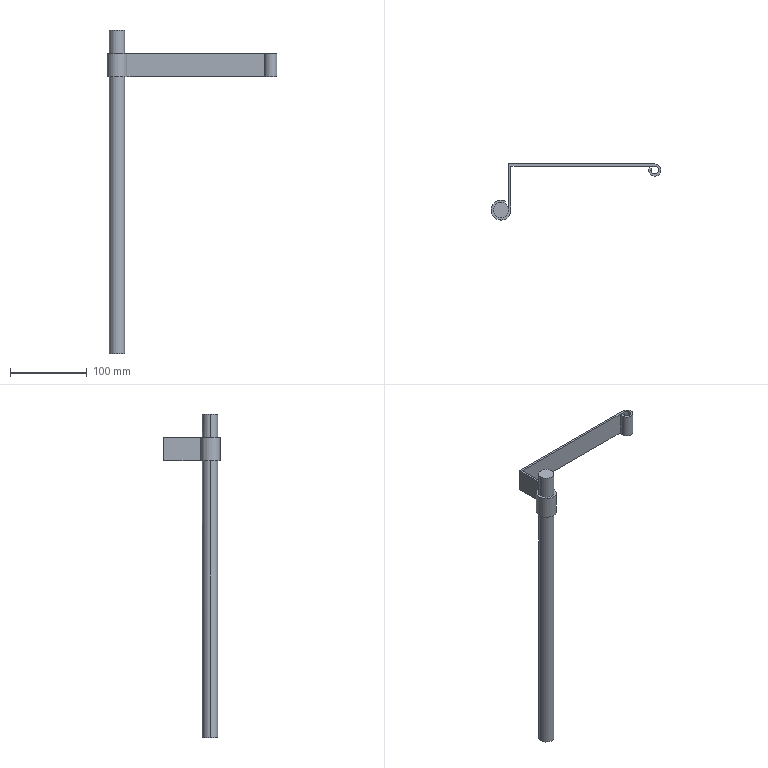Part | SolidWorks | features ICE 2, Revolution 1 | 1 solid | 20 faces | box 221 x 73 x 420 mm | volume 162659 mm3 | cylinder 10 | plane 10 | commonest cylinder face diameters 10 x3 16 x3 20 x3 26 x1
STEP:
#1=CARTESIAN_POINT('',(195.,52.,-15.));
#2=VERTEX_POINT('',#1);
#3=CARTESIAN_POINT('',(205.,52.,-15.));
#4=VERTEX_POINT('',#3);
#5=CARTESIAN_POINT('',(200.,52.,-15.));
#6=DIRECTION('',(0.,0.,1.));
#7=DIRECTION('',(-1.,0.,0.));
#8=AXIS2_PLACEMENT_3D('',#5,#6,#7);
#9=CIRCLE('',#8,5.);
#10=EDGE_CURVE('',#2,#4,#9,.T.);
#11=ORIENTED_EDGE('',*,*,#10,.F.);
#12=CARTESIAN_POINT('',(195.,52.,15.));
#13=VERTEX_POINT('',#12);
#14=CARTESIAN_POINT('',(195.,52.,-15.));
#15=DIRECTION('',(0.,0.,1.));
#16=VECTOR('',#15,1000.);
#17=LINE('',#14,#16);
#18=EDGE_CURVE('',#2,#13,#17,.T.);
#19=ORIENTED_EDGE('',*,*,#18,.T.);
#20=CARTESIAN_POINT('',(205.,52.,15.));
#21=VERTEX_POINT('',#20);
#22=CARTESIAN_POINT('',(200.,52.,15.));
#23=DIRECTION('',(0.,0.,1.));
#24=DIRECTION('',(-1.,0.,0.));
#25=AXIS2_PLACEMENT_3D('',#22,#23,#24);
#26=CIRCLE('',#25,5.);
#27=EDGE_CURVE('',#13,#21,#26,.T.);
#28=ORIENTED_EDGE('',*,*,#27,.T.);
#29=CARTESIAN_POINT('',(205.,52.,-15.));
#30=DIRECTION('',(0.,0.,1.));
#31=VECTOR('',#30,1000.);
#32=LINE('',#29,#31);
#33=EDGE_CURVE('',#4,#21,#32,.T.);
#34=ORIENTED_EDGE('',*,*,#33,.F.);
#35=EDGE_LOOP('',(#11,#19,#28,#34));
#36=FACE_OUTER_BOUND('',#35,.T.);
#37=CARTESIAN_POINT('',(200.,52.,-15.));
#38=DIRECTION('',(0.,0.,1.));
#39=DIRECTION('',(1.,0.,0.));
#40=AXIS2_PLACEMENT_3D('',#37,#38,#39);
#41=CYLINDRICAL_SURFACE('',#40,5.);
#42=ADVANCED_FACE('',(#36),#41,.F.);
#43=CARTESIAN_POINT('',(200.,57.,-15.));
#44=VERTEX_POINT('',#43);
#45=CARTESIAN_POINT('',(200.,52.,-15.));
#46=DIRECTION('',(0.,0.,1.));
#47=DIRECTION('',(-1.,0.,0.));
#48=AXIS2_PLACEMENT_3D('',#45,#46,#47);
#49=CIRCLE('',#48,5.);
#50=EDGE_CURVE('',#4,#44,#49,.T.);
#51=ORIENTED_EDGE('',*,*,#50,.F.);
#52=ORIENTED_EDGE('',*,*,#33,.T.);
#53=CARTESIAN_POINT('',(200.,57.,15.));
#54=VERTEX_POINT('',#53);
#55=CARTESIAN_POINT('',(200.,52.,15.));
#56=DIRECTION('',(0.,0.,1.));
#57=DIRECTION('',(-1.,0.,0.));
#58=AXIS2_PLACEMENT_3D('',#55,#56,#57);
#59=CIRCLE('',#58,5.);
#60=EDGE_CURVE('',#21,#54,#59,.T.);
#61=ORIENTED_EDGE('',*,*,#60,.T.);
#62=CARTESIAN_POINT('',(200.,57.,-15.));
#63=DIRECTION('',(0.,0.,1.));
#64=VECTOR('',#63,1000.);
#65=LINE('',#62,#64);
#66=EDGE_CURVE('',#44,#54,#65,.T.);
#67=ORIENTED_EDGE('',*,*,#66,.F.);
#68=EDGE_LOOP('',(#51,#52,#61,#67));
#69=FACE_OUTER_BOUND('',#68,.T.);
#70=CARTESIAN_POINT('',(200.,52.,-15.));
#71=DIRECTION('',(0.,0.,1.));
#72=DIRECTION('',(1.,0.,0.));
#73=AXIS2_PLACEMENT_3D('',#70,#71,#72);
#74=CYLINDRICAL_SURFACE('',#73,5.);
#75=ADVANCED_FACE('',(#69),#74,.F.);
#76=CARTESIAN_POINT('',(192.,52.,-15.));
#77=VERTEX_POINT('',#76);
#78=CARTESIAN_POINT('',(193.072,56.,-15.));
#79=VERTEX_POINT('',#78);
#80=CARTESIAN_POINT('',(200.,52.,-15.));
#81=DIRECTION('',(0.,0.,-1.));
#82=DIRECTION('',(1.,0.,0.));
#83=AXIS2_PLACEMENT_3D('',#80,#81,#82);
#84=CIRCLE('',#83,8.);
#85=EDGE_CURVE('',#77,#79,#84,.T.);
#86=ORIENTED_EDGE('',*,*,#85,.F.);
#87=CARTESIAN_POINT('',(192.,52.,15.));
#88=VERTEX_POINT('',#87);
#89=CARTESIAN_POINT('',(192.,52.,-15.));
#90=DIRECTION('',(0.,0.,1.));
#91=VECTOR('',#90,1000.);
#92=LINE('',#89,#91);
#93=EDGE_CURVE('',#77,#88,#92,.T.);
#94=ORIENTED_EDGE('',*,*,#93,.T.);
#95=CARTESIAN_POINT('',(193.072,56.,15.));
#96=VERTEX_POINT('',#95);
#97=CARTESIAN_POINT('',(200.,52.,15.));
#98=DIRECTION('',(0.,0.,-1.));
#99=DIRECTION('',(1.,0.,0.));
#100=AXIS2_PLACEMENT_3D('',#97,#98,#99);
#101=CIRCLE('',#100,8.);
#102=EDGE_CURVE('',#88,#96,#101,.T.);
#103=ORIENTED_EDGE('',*,*,#102,.T.);
#104=CARTESIAN_POINT('',(193.072,56.,-15.));
#105=DIRECTION('',(0.,0.,1.));
#106=VECTOR('',#105,1000.);
#107=LINE('',#104,#106);
#108=EDGE_CURVE('',#79,#96,#107,.T.);
#109=ORIENTED_EDGE('',*,*,#108,.F.);
#110=EDGE_LOOP('',(#86,#94,#103,#109));
#111=FACE_OUTER_BOUND('',#110,.T.);
#112=CARTESIAN_POINT('',(200.,52.,-15.));
#113=DIRECTION('',(0.,0.,1.));
#114=DIRECTION('',(1.,0.,0.));
#115=AXIS2_PLACEMENT_3D('',#112,#113,#114);
#116=CYLINDRICAL_SURFACE('',#115,8.);
#117=ADVANCED_FACE('',(#111),#116,.T.);
#118=ORIENTED_EDGE('',*,*,#93,.F.);
#119=CARTESIAN_POINT('',(208.,52.,-15.));
#120=VERTEX_POINT('',#119);
#121=CARTESIAN_POINT('',(200.,52.,-15.));
#122=DIRECTION('',(0.,0.,-1.));
#123=DIRECTION('',(1.,0.,0.));
#124=AXIS2_PLACEMENT_3D('',#121,#122,#123);
#125=CIRCLE('',#124,8.);
#126=EDGE_CURVE('',#120,#77,#125,.T.);
#127=ORIENTED_EDGE('',*,*,#126,.F.);
#128=CARTESIAN_POINT('',(208.,52.,15.));
#129=VERTEX_POINT('',#128);
#130=CARTESIAN_POINT('',(208.,52.,-15.));
#131=DIRECTION('',(0.,0.,1.));
#132=VECTOR('',#131,1000.);
#133=LINE('',#130,#132);
#134=EDGE_CURVE('',#120,#129,#133,.T.);
#135=ORIENTED_EDGE('',*,*,#134,.T.);
#136=CARTESIAN_POINT('',(200.,52.,15.));
#137=DIRECTION('',(0.,0.,-1.));
#138=DIRECTION('',(1.,0.,0.));
#139=AXIS2_PLACEMENT_3D('',#136,#137,#138);
#140=CIRCLE('',#139,8.);
#141=EDGE_CURVE('',#129,#88,#140,.T.);
#142=ORIENTED_EDGE('',*,*,#141,.T.);
#143=EDGE_LOOP('',(#118,#127,#135,#142));
#144=FACE_OUTER_BOUND('',#143,.T.);
#145=CARTESIAN_POINT('',(200.,52.,-15.));
#146=DIRECTION('',(0.,0.,1.));
#147=DIRECTION('',(1.,0.,0.));
#148=AXIS2_PLACEMENT_3D('',#145,#146,#147);
#149=CYLINDRICAL_SURFACE('',#148,8.);
#150=ADVANCED_FACE('',(#144),#149,.T.);
#151=CARTESIAN_POINT('',(-10.,0.,-375.));
#152=VERTEX_POINT('',#151);
#153=CARTESIAN_POINT('',(10.,0.,-375.));
#154=VERTEX_POINT('',#153);
#155=CARTESIAN_POINT('',(0.,0.,-375.));
#156=DIRECTION('',(0.,0.,-1.));
#157=DIRECTION('',(-1.,0.,0.));
#158=AXIS2_PLACEMENT_3D('',#155,#156,#157);
#159=CIRCLE('',#158,10.);
#160=EDGE_CURVE('',#152,#154,#159,.T.);
#161=ORIENTED_EDGE('',*,*,#160,.F.);
#162=CARTESIAN_POINT('',(-10.,0.,-15.));
#163=VERTEX_POINT('',#162);
#164=CARTESIAN_POINT('',(-10.,0.,15.));
#165=DIRECTION('',(0.,0.,1.));
#166=VECTOR('',#165,1000.);
#167=LINE('',#164,#166);
#168=EDGE_CURVE('',#152,#163,#167,.T.);
#169=ORIENTED_EDGE('',*,*,#168,.T.);
#170=CARTESIAN_POINT('',(5.,8.66,-15.));
#171=VERTEX_POINT('',#170);
#172=CARTESIAN_POINT('',(0.,0.,-15.));
#173=DIRECTION('',(0.,0.,-1.));
#174=DIRECTION('',(-1.,0.,0.));
#175=AXIS2_PLACEMENT_3D('',#172,#173,#174);
#176=CIRCLE('',#175,10.);
#177=EDGE_CURVE('',#163,#171,#176,.T.);
#178=ORIENTED_EDGE('',*,*,#177,.T.);
#179=CARTESIAN_POINT('',(5.,8.66,15.));
#180=VERTEX_POINT('',#179);
#181=CARTESIAN_POINT('',(5.,8.66,-15.));
#182=DIRECTION('',(0.,0.,1.));
#183=VECTOR('',#182,1000.);
#184=LINE('',#181,#183);
#185=EDGE_CURVE('',#171,#180,#184,.T.);
#186=ORIENTED_EDGE('',*,*,#185,.T.);
#187=CARTESIAN_POINT('',(-10.,0.,15.));
#188=VERTEX_POINT('',#187);
#189=CARTESIAN_POINT('',(0.,0.,15.));
#190=DIRECTION('',(0.,0.,1.));
#191=DIRECTION('',(1.,0.,0.));
#192=AXIS2_PLACEMENT_3D('',#189,#190,#191);
#193=CIRCLE('',#192,10.);
#194=EDGE_CURVE('',#180,#188,#193,.T.);
#195=ORIENTED_EDGE('',*,*,#194,.T.);
#196=CARTESIAN_POINT('',(-10.,0.,45.));
#197=VERTEX_POINT('',#196);
#198=CARTESIAN_POINT('',(-10.,0.,15.));
#199=DIRECTION('',(0.,0.,1.));
#200=VECTOR('',#199,1000.);
#201=LINE('',#198,#200);
#202=EDGE_CURVE('',#188,#197,#201,.T.);
#203=ORIENTED_EDGE('',*,*,#202,.T.);
#204=CARTESIAN_POINT('',(10.,0.,45.));
#205=VERTEX_POINT('',#204);
#206=CARTESIAN_POINT('',(0.,0.,45.));
#207=DIRECTION('',(0.,0.,1.));
#208=DIRECTION('',(1.,0.,0.));
#209=AXIS2_PLACEMENT_3D('',#206,#207,#208);
#210=CIRCLE('',#209,10.);
#211=EDGE_CURVE('',#205,#197,#210,.T.);
#212=ORIENTED_EDGE('',*,*,#211,.F.);
#213=CARTESIAN_POINT('',(10.,0.,15.));
#214=VERTEX_POINT('',#213);
#215=CARTESIAN_POINT('',(10.,0.,15.));
#216=DIRECTION('',(0.,0.,1.));
#217=VECTOR('',#216,1000.);
#218=LINE('',#215,#217);
#219=EDGE_CURVE('',#214,#205,#218,.T.);
#220=ORIENTED_EDGE('',*,*,#219,.F.);
#221=CARTESIAN_POINT('',(10.,0.,-15.));
#222=VERTEX_POINT('',#221);
#223=CARTESIAN_POINT('',(10.,0.,-15.));
#224=DIRECTION('',(0.,0.,1.));
#225=VECTOR('',#224,1000.);
#226=LINE('',#223,#225);
#227=EDGE_CURVE('',#222,#214,#226,.T.);
#228=ORIENTED_EDGE('',*,*,#227,.F.);
#229=CARTESIAN_POINT('',(10.,0.,15.));
#230=DIRECTION('',(0.,0.,1.));
#231=VECTOR('',#230,1000.);
#232=LINE('',#229,#231);
#233=EDGE_CURVE('',#154,#222,#232,.T.);
#234=ORIENTED_EDGE('',*,*,#233,.F.);
#235=EDGE_LOOP('',(#161,#169,#178,#186,#195,#203,#212,#220,#228,#234));
#236=FACE_OUTER_BOUND('',#235,.T.);
#237=CARTESIAN_POINT('',(0.,0.,15.));
#238=DIRECTION('',(0.,0.,1.));
#239=DIRECTION('',(1.,0.,0.));
#240=AXIS2_PLACEMENT_3D('',#237,#238,#239);
#241=CYLINDRICAL_SURFACE('',#240,10.);
#242=ADVANCED_FACE('',(#236),#241,.T.);
#243=ORIENTED_EDGE('',*,*,#168,.F.);
#244=CARTESIAN_POINT('',(0.,0.,-375.));
#245=DIRECTION('',(0.,0.,-1.));
#246=DIRECTION('',(-1.,0.,0.));
#247=AXIS2_PLACEMENT_3D('',#244,#245,#246);
#248=CIRCLE('',#247,10.);
#249=EDGE_CURVE('',#154,#152,#248,.T.);
#250=ORIENTED_EDGE('',*,*,#249,.F.);
#251=ORIENTED_EDGE('',*,*,#233,.T.);
#252=CARTESIAN_POINT('',(0.,0.,-15.));
#253=DIRECTION('',(0.,0.,-1.));
#254=DIRECTION('',(-1.,0.,0.));
#255=AXIS2_PLACEMENT_3D('',#252,#253,#254);
#256=CIRCLE('',#255,10.);
#257=EDGE_CURVE('',#222,#163,#256,.T.);
#258=ORIENTED_EDGE('',*,*,#257,.T.);
#259=EDGE_LOOP('',(#243,#250,#251,#258));
#260=FACE_OUTER_BOUND('',#259,.T.);
#261=CARTESIAN_POINT('',(0.,0.,15.));
#262=DIRECTION('',(0.,0.,1.));
#263=DIRECTION('',(1.,0.,0.));
#264=AXIS2_PLACEMENT_3D('',#261,#262,#263);
#265=CYLINDRICAL_SURFACE('',#264,10.);
#266=ADVANCED_FACE('',(#260),#265,.T.);
#267=ORIENTED_EDGE('',*,*,#202,.F.);
#268=CARTESIAN_POINT('',(0.,0.,15.));
#269=DIRECTION('',(0.,0.,1.));
#270=DIRECTION('',(1.,0.,0.));
#271=AXIS2_PLACEMENT_3D('',#268,#269,#270);
#272=CIRCLE('',#271,10.);
#273=EDGE_CURVE('',#188,#214,#272,.T.);
#274=ORIENTED_EDGE('',*,*,#273,.T.);
#275=ORIENTED_EDGE('',*,*,#219,.T.);
#276=CARTESIAN_POINT('',(0.,0.,45.));
#277=DIRECTION('',(0.,0.,1.));
#278=DIRECTION('',(1.,0.,0.));
#279=AXIS2_PLACEMENT_3D('',#276,#277,#278);
#280=CIRCLE('',#279,10.);
#281=EDGE_CURVE('',#197,#205,#280,.T.);
#282=ORIENTED_EDGE('',*,*,#281,.F.);
#283=EDGE_LOOP('',(#267,#274,#275,#282));
#284=FACE_OUTER_BOUND('',#283,.T.);
#285=CARTESIAN_POINT('',(0.,0.,15.));
#286=DIRECTION('',(0.,0.,1.));
#287=DIRECTION('',(1.,0.,0.));
#288=AXIS2_PLACEMENT_3D('',#285,#286,#287);
#289=CYLINDRICAL_SURFACE('',#288,10.);
#290=ADVANCED_FACE('',(#284),#289,.T.);
#291=ORIENTED_EDGE('',*,*,#211,.T.);
#292=ORIENTED_EDGE('',*,*,#281,.T.);
#293=EDGE_LOOP('',(#291,#292));
#294=FACE_OUTER_BOUND('',#293,.T.);
#295=CARTESIAN_POINT('',(0.,0.,45.));
#296=DIRECTION('',(0.,0.,1.));
#297=DIRECTION('',(1.,0.,0.));
#298=AXIS2_PLACEMENT_3D('',#295,#296,#297);
#299=PLANE('',#298);
#300=ADVANCED_FACE('',(#294),#299,.T.);
#301=ORIENTED_EDGE('',*,*,#194,.F.);
#302=CARTESIAN_POINT('',(6.5,11.258,15.));
#303=VERTEX_POINT('',#302);
#304=CARTESIAN_POINT('',(5.,8.66,15.));
#305=DIRECTION('',(-0.5,-0.866,0.));
#306=VECTOR('',#305,1000.);
#307=LINE('',#304,#306);
#308=EDGE_CURVE('',#303,#180,#307,.T.);
#309=ORIENTED_EDGE('',*,*,#308,.F.);
#310=CARTESIAN_POINT('',(13.,0.,15.));
#311=VERTEX_POINT('',#310);
#312=CARTESIAN_POINT('',(0.,0.,15.));
#313=DIRECTION('',(0.,0.,-1.));
#314=DIRECTION('',(1.,0.,0.));
#315=AXIS2_PLACEMENT_3D('',#312,#313,#314);
#316=CIRCLE('',#315,13.);
#317=EDGE_CURVE('',#311,#303,#316,.T.);
#318=ORIENTED_EDGE('',*,*,#317,.F.);
#319=CARTESIAN_POINT('',(13.,57.,15.));
#320=VERTEX_POINT('',#319);
#321=CARTESIAN_POINT('',(13.,0.,15.));
#322=DIRECTION('',(0.,-1.,0.));
#323=VECTOR('',#322,1000.);
#324=LINE('',#321,#323);
#325=EDGE_CURVE('',#320,#311,#324,.T.);
#326=ORIENTED_EDGE('',*,*,#325,.F.);
#327=CARTESIAN_POINT('',(13.,57.,15.));
#328=DIRECTION('',(-1.,0.,0.));
#329=VECTOR('',#328,1000.);
#330=LINE('',#327,#329);
#331=EDGE_CURVE('',#54,#320,#330,.T.);
#332=ORIENTED_EDGE('',*,*,#331,.F.);
#333=ORIENTED_EDGE('',*,*,#60,.F.);
#334=ORIENTED_EDGE('',*,*,#27,.F.);
#335=CARTESIAN_POINT('',(195.67,54.5,15.));
#336=VERTEX_POINT('',#335);
#337=CARTESIAN_POINT('',(200.,52.,15.));
#338=DIRECTION('',(0.,0.,1.));
#339=DIRECTION('',(-1.,0.,0.));
#340=AXIS2_PLACEMENT_3D('',#337,#338,#339);
#341=CIRCLE('',#340,5.);
#342=EDGE_CURVE('',#336,#13,#341,.T.);
#343=ORIENTED_EDGE('',*,*,#342,.F.);
#344=CARTESIAN_POINT('',(195.67,54.5,15.));
#345=DIRECTION('',(0.866,-0.5,0.));
#346=VECTOR('',#345,1000.);
#347=LINE('',#344,#346);
#348=EDGE_CURVE('',#96,#336,#347,.T.);
#349=ORIENTED_EDGE('',*,*,#348,.F.);
#350=ORIENTED_EDGE('',*,*,#102,.F.);
#351=ORIENTED_EDGE('',*,*,#141,.F.);
#352=CARTESIAN_POINT('',(200.,60.,15.));
#353=VERTEX_POINT('',#352);
#354=CARTESIAN_POINT('',(200.,52.,15.));
#355=DIRECTION('',(0.,0.,-1.));
#356=DIRECTION('',(1.,0.,0.));
#357=AXIS2_PLACEMENT_3D('',#354,#355,#356);
#358=CIRCLE('',#357,8.);
#359=EDGE_CURVE('',#353,#129,#358,.T.);
#360=ORIENTED_EDGE('',*,*,#359,.F.);
#361=CARTESIAN_POINT('',(10.,60.,15.));
#362=VERTEX_POINT('',#361);
#363=CARTESIAN_POINT('',(200.,60.,15.));
#364=DIRECTION('',(1.,0.,0.));
#365=VECTOR('',#364,1000.);
#366=LINE('',#363,#365);
#367=EDGE_CURVE('',#362,#353,#366,.T.);
#368=ORIENTED_EDGE('',*,*,#367,.F.);
#369=CARTESIAN_POINT('',(10.,60.,15.));
#370=DIRECTION('',(0.,1.,0.));
#371=VECTOR('',#370,1000.);
#372=LINE('',#369,#371);
#373=EDGE_CURVE('',#214,#362,#372,.T.);
#374=ORIENTED_EDGE('',*,*,#373,.F.);
#375=ORIENTED_EDGE('',*,*,#273,.F.);
#376=EDGE_LOOP('',(#301,#309,#318,#326,#332,#333,#334,#343,#349,#350,#351,#360,#368,#374,#375));
#377=FACE_OUTER_BOUND('',#376,.T.);
#378=CARTESIAN_POINT('',(0.,0.,15.));
#379=DIRECTION('',(0.,0.,1.));
#380=DIRECTION('',(1.,0.,0.));
#381=AXIS2_PLACEMENT_3D('',#378,#379,#380);
#382=PLANE('',#381);
#383=ADVANCED_FACE('',(#377),#382,.T.);
#384=ORIENTED_EDGE('',*,*,#373,.T.);
#385=CARTESIAN_POINT('',(10.,60.,-15.));
#386=VERTEX_POINT('',#385);
#387=CARTESIAN_POINT('',(10.,60.,-15.));
#388=DIRECTION('',(0.,0.,1.));
#389=VECTOR('',#388,1000.);
#390=LINE('',#387,#389);
#391=EDGE_CURVE('',#386,#362,#390,.T.);
#392=ORIENTED_EDGE('',*,*,#391,.F.);
#393=CARTESIAN_POINT('',(10.,60.,-15.));
#394=DIRECTION('',(0.,1.,0.));
#395=VECTOR('',#394,1000.);
#396=LINE('',#393,#395);
#397=EDGE_CURVE('',#222,#386,#396,.T.);
#398=ORIENTED_EDGE('',*,*,#397,.F.);
#399=ORIENTED_EDGE('',*,*,#227,.T.);
#400=EDGE_LOOP('',(#384,#392,#398,#399));
#401=FACE_OUTER_BOUND('',#400,.T.);
#402=CARTESIAN_POINT('',(10.,60.,-15.));
#403=DIRECTION('',(1.,0.,0.));
#404=DIRECTION('',(0.,0.,-1.));
#405=AXIS2_PLACEMENT_3D('',#402,#403,#404);
#406=PLANE('',#405);
#407=ADVANCED_FACE('',(#401),#406,.F.);
#408=ORIENTED_EDGE('',*,*,#367,.T.);
#409=CARTESIAN_POINT('',(200.,60.,-15.));
#410=VERTEX_POINT('',#409);
#411=CARTESIAN_POINT('',(200.,60.,-15.));
#412=DIRECTION('',(0.,0.,1.));
#413=VECTOR('',#412,1000.);
#414=LINE('',#411,#413);
#415=EDGE_CURVE('',#410,#353,#414,.T.);
#416=ORIENTED_EDGE('',*,*,#415,.F.);
#417=CARTESIAN_POINT('',(200.,60.,-15.));
#418=DIRECTION('',(1.,0.,0.));
#419=VECTOR('',#418,1000.);
#420=LINE('',#417,#419);
#421=EDGE_CURVE('',#386,#410,#420,.T.);
#422=ORIENTED_EDGE('',*,*,#421,.F.);
#423=ORIENTED_EDGE('',*,*,#391,.T.);
#424=EDGE_LOOP('',(#408,#416,#422,#423));
#425=FACE_OUTER_BOUND('',#424,.T.);
#426=CARTESIAN_POINT('',(200.,60.,-15.));
#427=DIRECTION('',(0.,-1.,0.));
#428=DIRECTION('',(0.,0.,-1.));
#429=AXIS2_PLACEMENT_3D('',#426,#427,#428);
#430=PLANE('',#429);
#431=ADVANCED_FACE('',(#425),#430,.F.);
#432=ORIENTED_EDGE('',*,*,#134,.F.);
#433=CARTESIAN_POINT('',(200.,52.,-15.));
#434=DIRECTION('',(0.,0.,-1.));
#435=DIRECTION('',(1.,0.,0.));
#436=AXIS2_PLACEMENT_3D('',#433,#434,#435);
#437=CIRCLE('',#436,8.);
#438=EDGE_CURVE('',#410,#120,#437,.T.);
#439=ORIENTED_EDGE('',*,*,#438,.F.);
#440=ORIENTED_EDGE('',*,*,#415,.T.);
#441=ORIENTED_EDGE('',*,*,#359,.T.);
#442=EDGE_LOOP('',(#432,#439,#440,#441));
#443=FACE_OUTER_BOUND('',#442,.T.);
#444=CARTESIAN_POINT('',(200.,52.,-15.));
#445=DIRECTION('',(0.,0.,1.));
#446=DIRECTION('',(1.,0.,0.));
#447=AXIS2_PLACEMENT_3D('',#444,#445,#446);
#448=CYLINDRICAL_SURFACE('',#447,8.);
#449=ADVANCED_FACE('',(#443),#448,.T.);
#450=ORIENTED_EDGE('',*,*,#348,.T.);
#451=CARTESIAN_POINT('',(195.67,54.5,-15.));
#452=VERTEX_POINT('',#451);
#453=CARTESIAN_POINT('',(195.67,54.5,-15.));
#454=DIRECTION('',(0.,0.,1.));
#455=VECTOR('',#454,1000.);
#456=LINE('',#453,#455);
#457=EDGE_CURVE('',#452,#336,#456,.T.);
#458=ORIENTED_EDGE('',*,*,#457,.F.);
#459=CARTESIAN_POINT('',(195.67,54.5,-15.));
#460=DIRECTION('',(0.866,-0.5,0.));
#461=VECTOR('',#460,1000.);
#462=LINE('',#459,#461);
#463=EDGE_CURVE('',#79,#452,#462,.T.);
#464=ORIENTED_EDGE('',*,*,#463,.F.);
#465=ORIENTED_EDGE('',*,*,#108,.T.);
#466=EDGE_LOOP('',(#450,#458,#464,#465));
#467=FACE_OUTER_BOUND('',#466,.T.);
#468=CARTESIAN_POINT('',(195.67,54.5,-15.));
#469=DIRECTION('',(-0.5,-0.866,0.));
#470=DIRECTION('',(0.866,-0.5,0.));
#471=AXIS2_PLACEMENT_3D('',#468,#469,#470);
#472=PLANE('',#471);
#473=ADVANCED_FACE('',(#467),#472,.F.);
#474=ORIENTED_EDGE('',*,*,#18,.F.);
#475=CARTESIAN_POINT('',(200.,52.,-15.));
#476=DIRECTION('',(0.,0.,1.));
#477=DIRECTION('',(-1.,0.,0.));
#478=AXIS2_PLACEMENT_3D('',#475,#476,#477);
#479=CIRCLE('',#478,5.);
#480=EDGE_CURVE('',#452,#2,#479,.T.);
#481=ORIENTED_EDGE('',*,*,#480,.F.);
#482=ORIENTED_EDGE('',*,*,#457,.T.);
#483=ORIENTED_EDGE('',*,*,#342,.T.);
#484=EDGE_LOOP('',(#474,#481,#482,#483));
#485=FACE_OUTER_BOUND('',#484,.T.);
#486=CARTESIAN_POINT('',(200.,52.,-15.));
#487=DIRECTION('',(0.,0.,1.));
#488=DIRECTION('',(1.,0.,0.));
#489=AXIS2_PLACEMENT_3D('',#486,#487,#488);
#490=CYLINDRICAL_SURFACE('',#489,5.);
#491=ADVANCED_FACE('',(#485),#490,.F.);
#492=ORIENTED_EDGE('',*,*,#331,.T.);
#493=CARTESIAN_POINT('',(13.,57.,-15.));
#494=VERTEX_POINT('',#493);
#495=CARTESIAN_POINT('',(13.,57.,-15.));
#496=DIRECTION('',(0.,0.,1.));
#497=VECTOR('',#496,1000.);
#498=LINE('',#495,#497);
#499=EDGE_CURVE('',#494,#320,#498,.T.);
#500=ORIENTED_EDGE('',*,*,#499,.F.);
#501=CARTESIAN_POINT('',(13.,57.,-15.));
#502=DIRECTION('',(-1.,0.,0.));
#503=VECTOR('',#502,1000.);
#504=LINE('',#501,#503);
#505=EDGE_CURVE('',#44,#494,#504,.T.);
#506=ORIENTED_EDGE('',*,*,#505,.F.);
#507=ORIENTED_EDGE('',*,*,#66,.T.);
#508=EDGE_LOOP('',(#492,#500,#506,#507));
#509=FACE_OUTER_BOUND('',#508,.T.);
#510=CARTESIAN_POINT('',(13.,57.,-15.));
#511=DIRECTION('',(0.,1.,0.));
#512=DIRECTION('',(0.,0.,1.));
#513=AXIS2_PLACEMENT_3D('',#510,#511,#512);
#514=PLANE('',#513);
#515=ADVANCED_FACE('',(#509),#514,.F.);
#516=ORIENTED_EDGE('',*,*,#325,.T.);
#517=CARTESIAN_POINT('',(13.,0.,-15.));
#518=VERTEX_POINT('',#517);
#519=CARTESIAN_POINT('',(13.,0.,-15.));
#520=DIRECTION('',(0.,0.,1.));
#521=VECTOR('',#520,1000.);
#522=LINE('',#519,#521);
#523=EDGE_CURVE('',#518,#311,#522,.T.);
#524=ORIENTED_EDGE('',*,*,#523,.F.);
#525=CARTESIAN_POINT('',(13.,0.,-15.));
#526=DIRECTION('',(0.,-1.,0.));
#527=VECTOR('',#526,1000.);
#528=LINE('',#525,#527);
#529=EDGE_CURVE('',#494,#518,#528,.T.);
#530=ORIENTED_EDGE('',*,*,#529,.F.);
#531=ORIENTED_EDGE('',*,*,#499,.T.);
#532=EDGE_LOOP('',(#516,#524,#530,#531));
#533=FACE_OUTER_BOUND('',#532,.T.);
#534=CARTESIAN_POINT('',(13.,0.,-15.));
#535=DIRECTION('',(-1.,0.,0.));
#536=DIRECTION('',(0.,0.,1.));
#537=AXIS2_PLACEMENT_3D('',#534,#535,#536);
#538=PLANE('',#537);
#539=ADVANCED_FACE('',(#533),#538,.F.);
#540=ORIENTED_EDGE('',*,*,#317,.T.);
#541=CARTESIAN_POINT('',(6.5,11.258,-15.));
#542=VERTEX_POINT('',#541);
#543=CARTESIAN_POINT('',(6.5,11.258,-15.));
#544=DIRECTION('',(0.,0.,1.));
#545=VECTOR('',#544,1000.);
#546=LINE('',#543,#545);
#547=EDGE_CURVE('',#542,#303,#546,.T.);
#548=ORIENTED_EDGE('',*,*,#547,.F.);
#549=CARTESIAN_POINT('',(0.,0.,-15.));
#550=DIRECTION('',(0.,0.,-1.));
#551=DIRECTION('',(1.,0.,0.));
#552=AXIS2_PLACEMENT_3D('',#549,#550,#551);
#553=CIRCLE('',#552,13.);
#554=EDGE_CURVE('',#518,#542,#553,.T.);
#555=ORIENTED_EDGE('',*,*,#554,.F.);
#556=ORIENTED_EDGE('',*,*,#523,.T.);
#557=EDGE_LOOP('',(#540,#548,#555,#556));
#558=FACE_OUTER_BOUND('',#557,.T.);
#559=CARTESIAN_POINT('',(0.,0.,-15.));
#560=DIRECTION('',(0.,0.,1.));
#561=DIRECTION('',(1.,0.,0.));
#562=AXIS2_PLACEMENT_3D('',#559,#560,#561);
#563=CYLINDRICAL_SURFACE('',#562,13.);
#564=ADVANCED_FACE('',(#558),#563,.T.);
#565=ORIENTED_EDGE('',*,*,#308,.T.);
#566=ORIENTED_EDGE('',*,*,#185,.F.);
#567=CARTESIAN_POINT('',(5.,8.66,-15.));
#568=DIRECTION('',(-0.5,-0.866,0.));
#569=VECTOR('',#568,1000.);
#570=LINE('',#567,#569);
#571=EDGE_CURVE('',#542,#171,#570,.T.);
#572=ORIENTED_EDGE('',*,*,#571,.F.);
#573=ORIENTED_EDGE('',*,*,#547,.T.);
#574=EDGE_LOOP('',(#565,#566,#572,#573));
#575=FACE_OUTER_BOUND('',#574,.T.);
#576=CARTESIAN_POINT('',(5.,8.66,-15.));
#577=DIRECTION('',(-0.866,0.5,0.));
#578=DIRECTION('',(-0.5,-0.866,0.));
#579=AXIS2_PLACEMENT_3D('',#576,#577,#578);
#580=PLANE('',#579);
#581=ADVANCED_FACE('',(#575),#580,.F.);
#582=ORIENTED_EDGE('',*,*,#257,.F.);
#583=ORIENTED_EDGE('',*,*,#397,.T.);
#584=ORIENTED_EDGE('',*,*,#421,.T.);
#585=ORIENTED_EDGE('',*,*,#438,.T.);
#586=ORIENTED_EDGE('',*,*,#126,.T.);
#587=ORIENTED_EDGE('',*,*,#85,.T.);
#588=ORIENTED_EDGE('',*,*,#463,.T.);
#589=ORIENTED_EDGE('',*,*,#480,.T.);
#590=ORIENTED_EDGE('',*,*,#10,.T.);
#591=ORIENTED_EDGE('',*,*,#50,.T.);
#592=ORIENTED_EDGE('',*,*,#505,.T.);
#593=ORIENTED_EDGE('',*,*,#529,.T.);
#594=ORIENTED_EDGE('',*,*,#554,.T.);
#595=ORIENTED_EDGE('',*,*,#571,.T.);
#596=ORIENTED_EDGE('',*,*,#177,.F.);
#597=EDGE_LOOP('',(#582,#583,#584,#585,#586,#587,#588,#589,#590,#591,#592,#593,#594,#595,#596));
#598=FACE_OUTER_BOUND('',#597,.T.);
#599=CARTESIAN_POINT('',(0.,0.,-15.));
#600=DIRECTION('',(0.,0.,1.));
#601=DIRECTION('',(1.,0.,0.));
#602=AXIS2_PLACEMENT_3D('',#599,#600,#601);
#603=PLANE('',#602);
#604=ADVANCED_FACE('',(#598),#603,.F.);
#605=ORIENTED_EDGE('',*,*,#249,.T.);
#606=ORIENTED_EDGE('',*,*,#160,.T.);
#607=EDGE_LOOP('',(#605,#606));
#608=FACE_OUTER_BOUND('',#607,.T.);
#609=CARTESIAN_POINT('',(0.,0.,-375.));
#610=DIRECTION('',(0.,0.,-1.));
#611=DIRECTION('',(-1.,0.,0.));
#612=AXIS2_PLACEMENT_3D('',#609,#610,#611);
#613=PLANE('',#612);
#614=ADVANCED_FACE('',(#608),#613,.T.);
#615=CLOSED_SHELL('',(#42,#75,#117,#150,#242,#266,#290,#300,#383,#407,#431,#449,#473,#491,#515,#539,#564,#581,#604,#614));
#616=MANIFOLD_SOLID_BREP('',#615);
#617=CARTESIAN_POINT('',(0.,0.,0.));
#618=DIRECTION('',(0.,0.,1.));
#619=DIRECTION('',(1.,0.,0.));
#620=AXIS2_PLACEMENT_3D('',#617,#618,#619);
#621=(LENGTH_UNIT()NAMED_UNIT(*)SI_UNIT(.MILLI.,.METRE.));
#622=UNCERTAINTY_MEASURE_WITH_UNIT(LENGTH_MEASURE(0.00001),#621,'','');
#623=(NAMED_UNIT(*)PLANE_ANGLE_UNIT()SI_UNIT($,.RADIAN.));
#624=(NAMED_UNIT(*)SI_UNIT($,.STERADIAN.)SOLID_ANGLE_UNIT());
#625=(GEOMETRIC_REPRESENTATION_CONTEXT(3)GLOBAL_UNCERTAINTY_ASSIGNED_CONTEXT((#622))GLOBAL_UNIT_ASSIGNED_CONTEXT((#621,#623,#624))REPRESENTATION_CONTEXT('',''));
#626=ADVANCED_BREP_SHAPE_REPRESENTATION('',(#616,#620),#625);